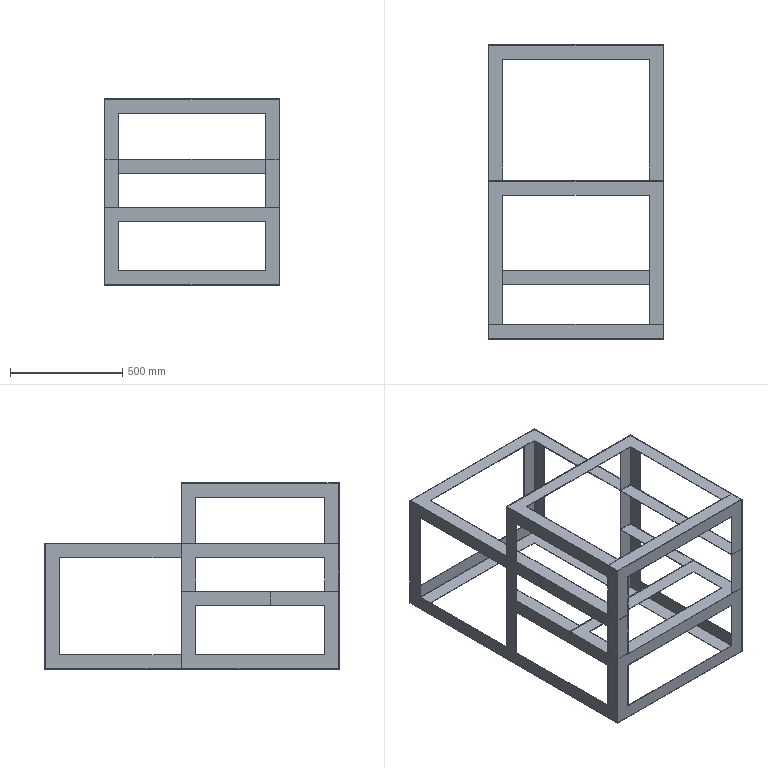Part | SolidWorks | features ICE 9, MirrorPattern 3, Extrusion 1 | 1 solid | 91 faces | box 780 x 1308 x 830 mm | volume 4147538 mm3 | plane 91